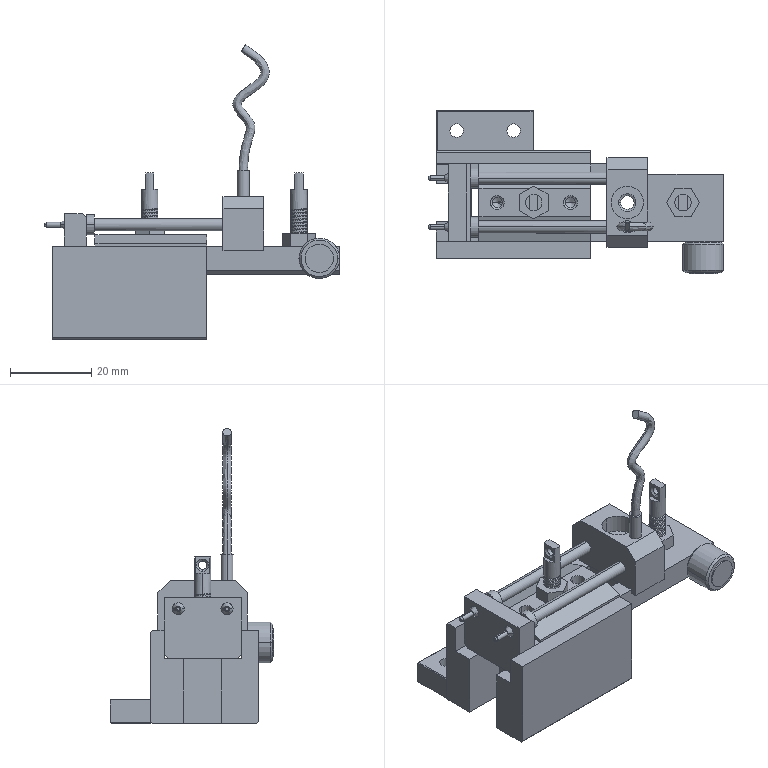Part | NX | 13 solids | 361 faces | box 72.65 x 40.25 x 72.548 mm | volume 31126 mm3 | cylinder 152 | plane 127 | cone 64 | spline 18 | commonest cylinder face diameters 4 x60 3 x26 3.3 x16 2.5 x14 3.5 x6 1 x4